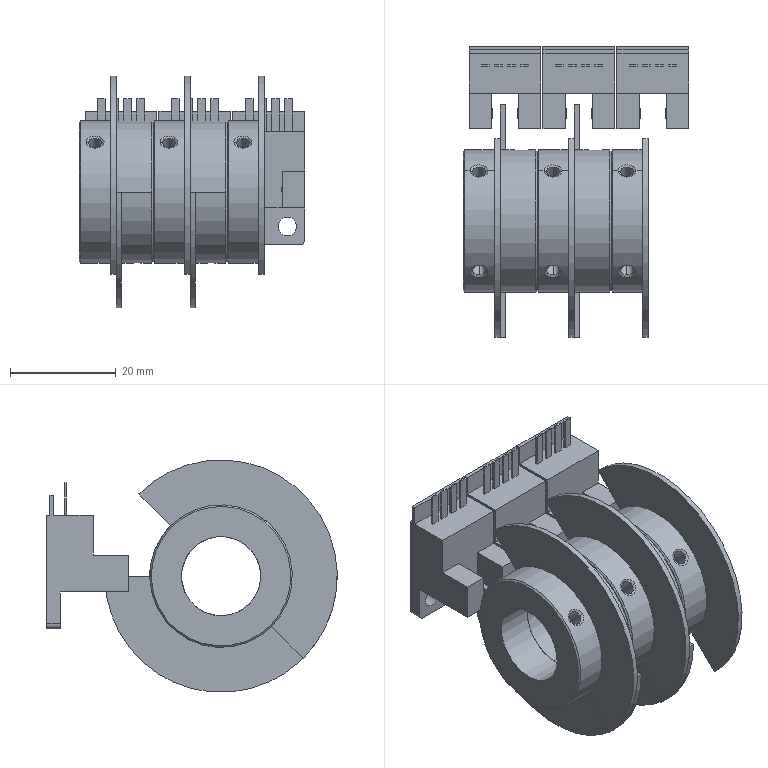Part | NX | 8 solids | 268 faces | box 42.7 x 55 x 44 mm | volume 23057 mm3 | plane 169 | cylinder 69 | spline 20 | cone 10 | commonest cylinder face diameters 2.5 x20 2 x12 3.5 x12 15 x10 27 x10 44 x5